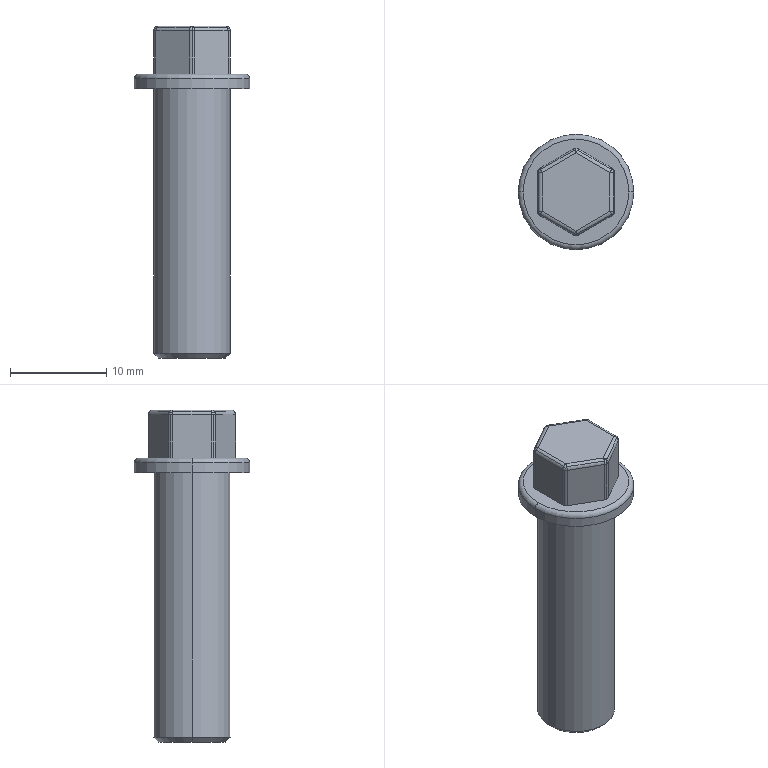Part | SolidWorks | features BaseBody 1 | 1 solid | 54 faces | box 12 x 12 x 34.5 mm | volume 1847 mm3 | cylinder 28 | sphere 12 | plane 10 | torus 2 | cone 2 | commonest cylinder face diameters 1 x24 8 x2 12 x2
STEP:
#1=CARTESIAN_POINT('',(-3.947,2.021,6.224));
#2=VERTEX_POINT('',#1);
#3=CARTESIAN_POINT('',(-4.,2.021,6.));
#4=VERTEX_POINT('',#3);
#5=CARTESIAN_POINT('',(-3.5,2.021,6.));
#6=DIRECTION('',(0.,-1.,0.));
#7=DIRECTION('',(0.,0.,1.));
#8=AXIS2_PLACEMENT_3D('',#5,#6,#7);
#9=CIRCLE('',#8,0.5);
#10=EDGE_CURVE('',#2,#4,#9,.T.);
#11=ORIENTED_EDGE('',*,*,#10,.F.);
#12=CARTESIAN_POINT('',(-3.724,2.408,6.224));
#13=VERTEX_POINT('',#12);
#14=CARTESIAN_POINT('',(-3.5,2.021,6.));
#15=DIRECTION('',(-0.433,0.25,-0.866));
#16=DIRECTION('',(-0.8944,0.,0.4472));
#17=AXIS2_PLACEMENT_3D('',#14,#15,#16);
#18=CIRCLE('',#17,0.5);
#19=EDGE_CURVE('',#2,#13,#18,.T.);
#20=ORIENTED_EDGE('',*,*,#19,.T.);
#21=CARTESIAN_POINT('',(-3.75,2.454,6.));
#22=VERTEX_POINT('',#21);
#23=CARTESIAN_POINT('',(-3.5,2.021,6.));
#24=DIRECTION('',(0.866,0.5,0.));
#25=DIRECTION('',(-0.5,0.866,0.));
#26=AXIS2_PLACEMENT_3D('',#23,#24,#25);
#27=CIRCLE('',#26,0.5);
#28=EDGE_CURVE('',#22,#13,#27,.T.);
#29=ORIENTED_EDGE('',*,*,#28,.F.);
#30=CARTESIAN_POINT('',(-3.933,2.271,6.));
#31=VERTEX_POINT('',#30);
#32=CARTESIAN_POINT('',(-3.5,2.021,6.));
#33=DIRECTION('',(0.,0.,-1.));
#34=DIRECTION('',(-1.,0.,0.));
#35=AXIS2_PLACEMENT_3D('',#32,#33,#34);
#36=CIRCLE('',#35,0.5);
#37=EDGE_CURVE('',#31,#22,#36,.T.);
#38=ORIENTED_EDGE('',*,*,#37,.F.);
#39=CARTESIAN_POINT('',(-3.5,2.021,6.));
#40=DIRECTION('',(0.,0.,-1.));
#41=DIRECTION('',(-1.,0.,0.));
#42=AXIS2_PLACEMENT_3D('',#39,#40,#41);
#43=CIRCLE('',#42,0.5);
#44=EDGE_CURVE('',#4,#31,#43,.T.);
#45=ORIENTED_EDGE('',*,*,#44,.F.);
#46=EDGE_LOOP('',(#11,#20,#29,#38,#45));
#47=FACE_OUTER_BOUND('',#46,.T.);
#48=CARTESIAN_POINT('',(-3.5,2.021,6.));
#49=DIRECTION('',(0.433,-0.25,0.866));
#50=DIRECTION('',(-0.75,0.433,0.5));
#51=AXIS2_PLACEMENT_3D('',#48,#49,#50);
#52=SPHERICAL_SURFACE('',#51,0.5);
#53=ADVANCED_FACE('',(#47),#52,.T.);
#54=ORIENTED_EDGE('',*,*,#44,.T.);
#55=CARTESIAN_POINT('',(-3.933,2.271,1.5));
#56=VERTEX_POINT('',#55);
#57=CARTESIAN_POINT('',(-3.933,2.271,1.5));
#58=DIRECTION('',(0.,0.,-1.));
#59=VECTOR('',#58,1000.);
#60=LINE('',#57,#59);
#61=EDGE_CURVE('',#31,#56,#60,.T.);
#62=ORIENTED_EDGE('',*,*,#61,.T.);
#63=CARTESIAN_POINT('',(-4.,2.021,1.5));
#64=VERTEX_POINT('',#63);
#65=CARTESIAN_POINT('',(-3.5,2.021,1.5));
#66=DIRECTION('',(0.,0.,1.));
#67=DIRECTION('',(-0.866,0.5,0.));
#68=AXIS2_PLACEMENT_3D('',#65,#66,#67);
#69=CIRCLE('',#68,0.5);
#70=EDGE_CURVE('',#56,#64,#69,.T.);
#71=ORIENTED_EDGE('',*,*,#70,.T.);
#72=CARTESIAN_POINT('',(-4.,2.021,1.5));
#73=DIRECTION('',(0.,0.,1.));
#74=VECTOR('',#73,1000.);
#75=LINE('',#72,#74);
#76=EDGE_CURVE('',#64,#4,#75,.T.);
#77=ORIENTED_EDGE('',*,*,#76,.T.);
#78=EDGE_LOOP('',(#54,#62,#71,#77));
#79=FACE_OUTER_BOUND('',#78,.T.);
#80=CARTESIAN_POINT('',(-3.5,2.021,1.5));
#81=DIRECTION('',(0.,0.,-1.));
#82=DIRECTION('',(-0.866,0.5,0.));
#83=AXIS2_PLACEMENT_3D('',#80,#81,#82);
#84=CYLINDRICAL_SURFACE('',#83,0.5);
#85=ADVANCED_FACE('',(#79),#84,.T.);
#86=CARTESIAN_POINT('',(-3.724,-2.408,6.224));
#87=VERTEX_POINT('',#86);
#88=CARTESIAN_POINT('',(-3.75,-2.454,6.));
#89=VERTEX_POINT('',#88);
#90=CARTESIAN_POINT('',(-3.5,-2.021,6.));
#91=DIRECTION('',(0.866,-0.5,0.));
#92=DIRECTION('',(0.,0.,1.));
#93=AXIS2_PLACEMENT_3D('',#90,#91,#92);
#94=CIRCLE('',#93,0.5);
#95=EDGE_CURVE('',#87,#89,#94,.T.);
#96=ORIENTED_EDGE('',*,*,#95,.F.);
#97=CARTESIAN_POINT('',(-3.947,-2.021,6.224));
#98=VERTEX_POINT('',#97);
#99=CARTESIAN_POINT('',(-3.5,-2.021,6.));
#100=DIRECTION('',(-0.433,-0.25,-0.866));
#101=DIRECTION('',(-0.8944,0.,0.4472));
#102=AXIS2_PLACEMENT_3D('',#99,#100,#101);
#103=CIRCLE('',#102,0.5);
#104=EDGE_CURVE('',#87,#98,#103,.T.);
#105=ORIENTED_EDGE('',*,*,#104,.T.);
#106=CARTESIAN_POINT('',(-4.,-2.021,6.));
#107=VERTEX_POINT('',#106);
#108=CARTESIAN_POINT('',(-3.5,-2.021,6.));
#109=DIRECTION('',(0.,1.,0.));
#110=DIRECTION('',(-1.,0.,0.));
#111=AXIS2_PLACEMENT_3D('',#108,#109,#110);
#112=CIRCLE('',#111,0.5);
#113=EDGE_CURVE('',#107,#98,#112,.T.);
#114=ORIENTED_EDGE('',*,*,#113,.F.);
#115=CARTESIAN_POINT('',(-3.933,-2.271,6.));
#116=VERTEX_POINT('',#115);
#117=CARTESIAN_POINT('',(-3.5,-2.021,6.));
#118=DIRECTION('',(0.,0.,-1.));
#119=DIRECTION('',(-0.5,-0.866,0.));
#120=AXIS2_PLACEMENT_3D('',#117,#118,#119);
#121=CIRCLE('',#120,0.5);
#122=EDGE_CURVE('',#116,#107,#121,.T.);
#123=ORIENTED_EDGE('',*,*,#122,.F.);
#124=CARTESIAN_POINT('',(-3.5,-2.021,6.));
#125=DIRECTION('',(0.,0.,-1.));
#126=DIRECTION('',(-0.5,-0.866,0.));
#127=AXIS2_PLACEMENT_3D('',#124,#125,#126);
#128=CIRCLE('',#127,0.5);
#129=EDGE_CURVE('',#89,#116,#128,.T.);
#130=ORIENTED_EDGE('',*,*,#129,.F.);
#131=EDGE_LOOP('',(#96,#105,#114,#123,#130));
#132=FACE_OUTER_BOUND('',#131,.T.);
#133=CARTESIAN_POINT('',(-3.5,-2.021,6.));
#134=DIRECTION('',(0.433,0.25,0.866));
#135=DIRECTION('',(-0.75,-0.433,0.5));
#136=AXIS2_PLACEMENT_3D('',#133,#134,#135);
#137=SPHERICAL_SURFACE('',#136,0.5);
#138=ADVANCED_FACE('',(#132),#137,.T.);
#139=ORIENTED_EDGE('',*,*,#129,.T.);
#140=CARTESIAN_POINT('',(-3.933,-2.271,1.5));
#141=VERTEX_POINT('',#140);
#142=CARTESIAN_POINT('',(-3.933,-2.271,1.5));
#143=DIRECTION('',(0.,0.,-1.));
#144=VECTOR('',#143,1000.);
#145=LINE('',#142,#144);
#146=EDGE_CURVE('',#116,#141,#145,.T.);
#147=ORIENTED_EDGE('',*,*,#146,.T.);
#148=CARTESIAN_POINT('',(-3.75,-2.454,1.5));
#149=VERTEX_POINT('',#148);
#150=CARTESIAN_POINT('',(-3.5,-2.021,1.5));
#151=DIRECTION('',(0.,0.,1.));
#152=DIRECTION('',(-0.866,-0.5,0.));
#153=AXIS2_PLACEMENT_3D('',#150,#151,#152);
#154=CIRCLE('',#153,0.5);
#155=EDGE_CURVE('',#141,#149,#154,.T.);
#156=ORIENTED_EDGE('',*,*,#155,.T.);
#157=CARTESIAN_POINT('',(-3.75,-2.454,1.5));
#158=DIRECTION('',(0.,0.,1.));
#159=VECTOR('',#158,1000.);
#160=LINE('',#157,#159);
#161=EDGE_CURVE('',#149,#89,#160,.T.);
#162=ORIENTED_EDGE('',*,*,#161,.T.);
#163=EDGE_LOOP('',(#139,#147,#156,#162));
#164=FACE_OUTER_BOUND('',#163,.T.);
#165=CARTESIAN_POINT('',(-3.5,-2.021,1.5));
#166=DIRECTION('',(0.,0.,-1.));
#167=DIRECTION('',(-0.866,-0.5,0.));
#168=AXIS2_PLACEMENT_3D('',#165,#166,#167);
#169=CYLINDRICAL_SURFACE('',#168,0.5);
#170=ADVANCED_FACE('',(#164),#169,.T.);
#171=CARTESIAN_POINT('',(0.,4.041,6.5));
#172=VERTEX_POINT('',#171);
#173=CARTESIAN_POINT('',(-0.1768,4.348,6.354));
#174=VERTEX_POINT('',#173);
#175=CARTESIAN_POINT('',(0.,4.041,6.));
#176=DIRECTION('',(-0.866,-0.5,0.));
#177=DIRECTION('',(0.,0.,1.));
#178=AXIS2_PLACEMENT_3D('',#175,#176,#177);
#179=CIRCLE('',#178,0.5);
#180=EDGE_CURVE('',#172,#174,#179,.T.);
#181=ORIENTED_EDGE('',*,*,#180,.F.);
#182=CARTESIAN_POINT('',(0.,4.541,6.));
#183=VERTEX_POINT('',#182);
#184=CARTESIAN_POINT('',(0.,4.041,6.));
#185=DIRECTION('',(-1.,0.,0.));
#186=DIRECTION('',(0.,-1.,0.));
#187=AXIS2_PLACEMENT_3D('',#184,#185,#186);
#188=CIRCLE('',#187,0.5);
#189=EDGE_CURVE('',#172,#183,#188,.T.);
#190=ORIENTED_EDGE('',*,*,#189,.T.);
#191=CARTESIAN_POINT('',(-0.25,4.474,6.));
#192=VERTEX_POINT('',#191);
#193=CARTESIAN_POINT('',(0.,4.041,6.));
#194=DIRECTION('',(0.,0.,-1.));
#195=DIRECTION('',(-0.5,0.866,0.));
#196=AXIS2_PLACEMENT_3D('',#193,#194,#195);
#197=CIRCLE('',#196,0.5);
#198=EDGE_CURVE('',#192,#183,#197,.T.);
#199=ORIENTED_EDGE('',*,*,#198,.F.);
#200=CARTESIAN_POINT('',(0.,4.041,6.));
#201=DIRECTION('',(-0.866,-0.5,0.));
#202=DIRECTION('',(0.,0.,1.));
#203=AXIS2_PLACEMENT_3D('',#200,#201,#202);
#204=CIRCLE('',#203,0.5);
#205=EDGE_CURVE('',#174,#192,#204,.T.);
#206=ORIENTED_EDGE('',*,*,#205,.F.);
#207=EDGE_LOOP('',(#181,#190,#199,#206));
#208=FACE_OUTER_BOUND('',#207,.T.);
#209=CARTESIAN_POINT('',(0.,4.041,6.));
#210=DIRECTION('',(1.,0.,0.));
#211=DIRECTION('',(0.,0.866,0.5));
#212=AXIS2_PLACEMENT_3D('',#209,#210,#211);
#213=SPHERICAL_SURFACE('',#212,0.5);
#214=ADVANCED_FACE('',(#208),#213,.T.);
#215=ORIENTED_EDGE('',*,*,#198,.T.);
#216=CARTESIAN_POINT('',(0.,4.541,1.5));
#217=VERTEX_POINT('',#216);
#218=CARTESIAN_POINT('',(0.,4.541,1.5));
#219=DIRECTION('',(0.,0.,-1.));
#220=VECTOR('',#219,1000.);
#221=LINE('',#218,#220);
#222=EDGE_CURVE('',#183,#217,#221,.T.);
#223=ORIENTED_EDGE('',*,*,#222,.T.);
#224=CARTESIAN_POINT('',(-0.25,4.474,1.5));
#225=VERTEX_POINT('',#224);
#226=CARTESIAN_POINT('',(0.,4.041,1.5));
#227=DIRECTION('',(0.,0.,1.));
#228=DIRECTION('',(0.,1.,0.));
#229=AXIS2_PLACEMENT_3D('',#226,#227,#228);
#230=CIRCLE('',#229,0.5);
#231=EDGE_CURVE('',#217,#225,#230,.T.);
#232=ORIENTED_EDGE('',*,*,#231,.T.);
#233=CARTESIAN_POINT('',(-0.25,4.474,1.5));
#234=DIRECTION('',(0.,0.,1.));
#235=VECTOR('',#234,1000.);
#236=LINE('',#233,#235);
#237=EDGE_CURVE('',#225,#192,#236,.T.);
#238=ORIENTED_EDGE('',*,*,#237,.T.);
#239=EDGE_LOOP('',(#215,#223,#232,#238));
#240=FACE_OUTER_BOUND('',#239,.T.);
#241=CARTESIAN_POINT('',(0.,4.041,1.5));
#242=DIRECTION('',(0.,0.,-1.));
#243=DIRECTION('',(0.,1.,0.));
#244=AXIS2_PLACEMENT_3D('',#241,#242,#243);
#245=CYLINDRICAL_SURFACE('',#244,0.5);
#246=ADVANCED_FACE('',(#240),#245,.T.);
#247=ORIENTED_EDGE('',*,*,#28,.T.);
#248=CARTESIAN_POINT('',(-3.677,2.327,6.354));
#249=VERTEX_POINT('',#248);
#250=CARTESIAN_POINT('',(-3.5,2.021,6.));
#251=DIRECTION('',(0.866,0.5,0.));
#252=DIRECTION('',(-0.5,0.866,0.));
#253=AXIS2_PLACEMENT_3D('',#250,#251,#252);
#254=CIRCLE('',#253,0.5);
#255=EDGE_CURVE('',#13,#249,#254,.T.);
#256=ORIENTED_EDGE('',*,*,#255,.T.);
#257=CARTESIAN_POINT('',(-0.9268,3.915,6.354));
#258=DIRECTION('',(0.866,0.5,0.));
#259=VECTOR('',#258,1000.);
#260=LINE('',#257,#259);
#261=EDGE_CURVE('',#249,#174,#260,.T.);
#262=ORIENTED_EDGE('',*,*,#261,.T.);
#263=ORIENTED_EDGE('',*,*,#205,.T.);
#264=CARTESIAN_POINT('',(-1.,4.041,6.));
#265=DIRECTION('',(-0.866,-0.5,0.));
#266=VECTOR('',#265,1000.);
#267=LINE('',#264,#266);
#268=EDGE_CURVE('',#192,#22,#267,.T.);
#269=ORIENTED_EDGE('',*,*,#268,.T.);
#270=EDGE_LOOP('',(#247,#256,#262,#263,#269));
#271=FACE_OUTER_BOUND('',#270,.T.);
#272=CARTESIAN_POINT('',(-0.75,3.608,6.));
#273=DIRECTION('',(0.866,0.5,0.));
#274=DIRECTION('',(-0.3536,0.6124,0.7071));
#275=AXIS2_PLACEMENT_3D('',#272,#273,#274);
#276=CYLINDRICAL_SURFACE('',#275,0.5);
#277=ADVANCED_FACE('',(#271),#276,.T.);
#278=CARTESIAN_POINT('',(0.,-4.541,6.));
#279=VERTEX_POINT('',#278);
#280=CARTESIAN_POINT('',(-0.25,-4.474,6.));
#281=VERTEX_POINT('',#280);
#282=CARTESIAN_POINT('',(0.,-4.041,6.));
#283=DIRECTION('',(0.,0.,-1.));
#284=DIRECTION('',(0.5,-0.866,0.));
#285=AXIS2_PLACEMENT_3D('',#282,#283,#284);
#286=CIRCLE('',#285,0.5);
#287=EDGE_CURVE('',#279,#281,#286,.T.);
#288=ORIENTED_EDGE('',*,*,#287,.F.);
#289=CARTESIAN_POINT('',(0.,-4.041,6.5));
#290=VERTEX_POINT('',#289);
#291=CARTESIAN_POINT('',(0.,-4.041,6.));
#292=DIRECTION('',(-1.,0.,0.));
#293=DIRECTION('',(0.,-1.,0.));
#294=AXIS2_PLACEMENT_3D('',#291,#292,#293);
#295=CIRCLE('',#294,0.5);
#296=EDGE_CURVE('',#279,#290,#295,.T.);
#297=ORIENTED_EDGE('',*,*,#296,.T.);
#298=CARTESIAN_POINT('',(-0.1768,-4.348,6.354));
#299=VERTEX_POINT('',#298);
#300=CARTESIAN_POINT('',(0.,-4.041,6.));
#301=DIRECTION('',(-0.866,0.5,0.));
#302=DIRECTION('',(-0.5,-0.866,0.));
#303=AXIS2_PLACEMENT_3D('',#300,#301,#302);
#304=CIRCLE('',#303,0.5);
#305=EDGE_CURVE('',#299,#290,#304,.T.);
#306=ORIENTED_EDGE('',*,*,#305,.F.);
#307=CARTESIAN_POINT('',(0.,-4.041,6.));
#308=DIRECTION('',(-0.866,0.5,0.));
#309=DIRECTION('',(-0.5,-0.866,0.));
#310=AXIS2_PLACEMENT_3D('',#307,#308,#309);
#311=CIRCLE('',#310,0.5);
#312=EDGE_CURVE('',#281,#299,#311,.T.);
#313=ORIENTED_EDGE('',*,*,#312,.F.);
#314=EDGE_LOOP('',(#288,#297,#306,#313));
#315=FACE_OUTER_BOUND('',#314,.T.);
#316=CARTESIAN_POINT('',(0.,-4.041,6.));
#317=DIRECTION('',(1.,0.,0.));
#318=DIRECTION('',(0.,-0.866,0.5));
#319=AXIS2_PLACEMENT_3D('',#316,#317,#318);
#320=SPHERICAL_SURFACE('',#319,0.5);
#321=ADVANCED_FACE('',(#315),#320,.T.);
#322=CARTESIAN_POINT('',(0.25,-4.474,6.));
#323=VERTEX_POINT('',#322);
#324=CARTESIAN_POINT('',(0.,-4.041,6.));
#325=DIRECTION('',(0.,0.,-1.));
#326=DIRECTION('',(0.5,-0.866,0.));
#327=AXIS2_PLACEMENT_3D('',#324,#325,#326);
#328=CIRCLE('',#327,0.5);
#329=EDGE_CURVE('',#323,#279,#328,.T.);
#330=ORIENTED_EDGE('',*,*,#329,.T.);
#331=CARTESIAN_POINT('',(0.,-4.541,1.5));
#332=VERTEX_POINT('',#331);
#333=CARTESIAN_POINT('',(0.,-4.541,1.5));
#334=DIRECTION('',(0.,0.,-1.));
#335=VECTOR('',#334,1000.);
#336=LINE('',#333,#335);
#337=EDGE_CURVE('',#279,#332,#336,.T.);
#338=ORIENTED_EDGE('',*,*,#337,.T.);
#339=CARTESIAN_POINT('',(0.25,-4.474,1.5));
#340=VERTEX_POINT('',#339);
#341=CARTESIAN_POINT('',(0.,-4.041,1.5));
#342=DIRECTION('',(0.,0.,1.));
#343=DIRECTION('',(0.,-1.,0.));
#344=AXIS2_PLACEMENT_3D('',#341,#342,#343);
#345=CIRCLE('',#344,0.5);
#346=EDGE_CURVE('',#332,#340,#345,.T.);
#347=ORIENTED_EDGE('',*,*,#346,.T.);
#348=CARTESIAN_POINT('',(0.25,-4.474,1.5));
#349=DIRECTION('',(0.,0.,1.));
#350=VECTOR('',#349,1000.);
#351=LINE('',#348,#350);
#352=EDGE_CURVE('',#340,#323,#351,.T.);
#353=ORIENTED_EDGE('',*,*,#352,.T.);
#354=EDGE_LOOP('',(#330,#338,#347,#353));
#355=FACE_OUTER_BOUND('',#354,.T.);
#356=CARTESIAN_POINT('',(0.,-4.041,1.5));
#357=DIRECTION('',(0.,0.,-1.));
#358=DIRECTION('',(0.,-1.,0.));
#359=AXIS2_PLACEMENT_3D('',#356,#357,#358);
#360=CYLINDRICAL_SURFACE('',#359,0.5);
#361=ADVANCED_FACE('',(#355),#360,.T.);
#362=CARTESIAN_POINT('',(3.724,2.408,6.224));
#363=VERTEX_POINT('',#362);
#364=CARTESIAN_POINT('',(3.75,2.454,6.));
#365=VERTEX_POINT('',#364);
#366=CARTESIAN_POINT('',(3.5,2.021,6.));
#367=DIRECTION('',(-0.866,0.5,0.));
#368=DIRECTION('',(0.,0.,1.));
#369=AXIS2_PLACEMENT_3D('',#366,#367,#368);
#370=CIRCLE('',#369,0.5);
#371=EDGE_CURVE('',#363,#365,#370,.T.);
#372=ORIENTED_EDGE('',*,*,#371,.F.);
#373=CARTESIAN_POINT('',(3.947,2.021,6.224));
#374=VERTEX_POINT('',#373);
#375=CARTESIAN_POINT('',(3.5,2.021,6.));
#376=DIRECTION('',(0.433,0.25,-0.866));
#377=DIRECTION('',(-0.8944,0.,-0.4472));
#378=AXIS2_PLACEMENT_3D('',#375,#376,#377);
#379=CIRCLE('',#378,0.5);
#380=EDGE_CURVE('',#363,#374,#379,.T.);
#381=ORIENTED_EDGE('',*,*,#380,.T.);
#382=CARTESIAN_POINT('',(4.,2.021,6.));
#383=VERTEX_POINT('',#382);
#384=CARTESIAN_POINT('',(3.5,2.021,6.));
#385=DIRECTION('',(0.,-1.,0.));
#386=DIRECTION('',(1.,0.,0.));
#387=AXIS2_PLACEMENT_3D('',#384,#385,#386);
#388=CIRCLE('',#387,0.5);
#389=EDGE_CURVE('',#383,#374,#388,.T.);
#390=ORIENTED_EDGE('',*,*,#389,.F.);
#391=CARTESIAN_POINT('',(3.933,2.271,6.));
#392=VERTEX_POINT('',#391);
#393=CARTESIAN_POINT('',(3.5,2.021,6.));
#394=DIRECTION('',(0.,0.,-1.));
#395=DIRECTION('',(0.5,0.866,0.));
#396=AXIS2_PLACEMENT_3D('',#393,#394,#395);
#397=CIRCLE('',#396,0.5);
#398=EDGE_CURVE('',#392,#383,#397,.T.);
#399=ORIENTED_EDGE('',*,*,#398,.F.);
#400=CARTESIAN_POINT('',(3.5,2.021,6.));
#401=DIRECTION('',(0.,0.,-1.));
#402=DIRECTION('',(0.5,0.866,0.));
#403=AXIS2_PLACEMENT_3D('',#400,#401,#402);
#404=CIRCLE('',#403,0.5);
#405=EDGE_CURVE('',#365,#392,#404,.T.);
#406=ORIENTED_EDGE('',*,*,#405,.F.);
#407=EDGE_LOOP('',(#372,#381,#390,#399,#406));
#408=FACE_OUTER_BOUND('',#407,.T.);
#409=CARTESIAN_POINT('',(3.5,2.021,6.));
#410=DIRECTION('',(-0.433,-0.25,0.866));
#411=DIRECTION('',(0.75,0.433,0.5));
#412=AXIS2_PLACEMENT_3D('',#409,#410,#411);
#413=SPHERICAL_SURFACE('',#412,0.5);
#414=ADVANCED_FACE('',(#408),#413,.T.);
#415=ORIENTED_EDGE('',*,*,#405,.T.);
#416=CARTESIAN_POINT('',(3.933,2.271,1.5));
#417=VERTEX_POINT('',#416);
#418=CARTESIAN_POINT('',(3.933,2.271,1.5));
#419=DIRECTION('',(0.,0.,-1.));
#420=VECTOR('',#419,1000.);
#421=LINE('',#418,#420);
#422=EDGE_CURVE('',#392,#417,#421,.T.);
#423=ORIENTED_EDGE('',*,*,#422,.T.);
#424=CARTESIAN_POINT('',(3.75,2.454,1.5));
#425=VERTEX_POINT('',#424);
#426=CARTESIAN_POINT('',(3.5,2.021,1.5));
#427=DIRECTION('',(0.,0.,1.));
#428=DIRECTION('',(0.866,0.5,0.));
#429=AXIS2_PLACEMENT_3D('',#426,#427,#428);
#430=CIRCLE('',#429,0.5);
#431=EDGE_CURVE('',#417,#425,#430,.T.);
#432=ORIENTED_EDGE('',*,*,#431,.T.);
#433=CARTESIAN_POINT('',(3.75,2.454,1.5));
#434=DIRECTION('',(0.,0.,1.));
#435=VECTOR('',#434,1000.);
#436=LINE('',#433,#435);
#437=EDGE_CURVE('',#425,#365,#436,.T.);
#438=ORIENTED_EDGE('',*,*,#437,.T.);
#439=EDGE_LOOP('',(#415,#423,#432,#438));
#440=FACE_OUTER_BOUND('',#439,.T.);
#441=CARTESIAN_POINT('',(3.5,2.021,1.5));
#442=DIRECTION('',(0.,0.,-1.));
#443=DIRECTION('',(0.866,0.5,0.));
#444=AXIS2_PLACEMENT_3D('',#441,#442,#443);
#445=CYLINDRICAL_SURFACE('',#444,0.5);
#446=ADVANCED_FACE('',(#440),#445,.T.);
#447=CARTESIAN_POINT('',(0.25,4.474,6.));
#448=VERTEX_POINT('',#447);
#449=CARTESIAN_POINT('',(0.1768,4.348,6.354));
#450=VERTEX_POINT('',#449);
#451=CARTESIAN_POINT('',(0.,4.041,6.));
#452=DIRECTION('',(0.866,-0.5,0.));
#453=DIRECTION('',(0.5,0.866,0.));
#454=AXIS2_PLACEMENT_3D('',#451,#452,#453);
#455=CIRCLE('',#454,0.5);
#456=EDGE_CURVE('',#448,#450,#455,.T.);
#457=ORIENTED_EDGE('',*,*,#456,.T.);
#458=CARTESIAN_POINT('',(3.677,2.327,6.354));
#459=VERTEX_POINT('',#458);
#460=CARTESIAN_POINT('',(2.927,2.76,6.354));
#461=DIRECTION('',(0.866,-0.5,0.));
#462=VECTOR('',#461,1000.);
#463=LINE('',#460,#462);
#464=EDGE_CURVE('',#450,#459,#463,.T.);
#465=ORIENTED_EDGE('',*,*,#464,.T.);
#466=CARTESIAN_POINT('',(3.5,2.021,6.));
#467=DIRECTION('',(-0.866,0.5,0.));
#468=DIRECTION('',(0.,0.,1.));
#469=AXIS2_PLACEMENT_3D('',#466,#467,#468);
#470=CIRCLE('',#469,0.5);
#471=EDGE_CURVE('',#459,#363,#470,.T.);
#472=ORIENTED_EDGE('',*,*,#471,.T.);
#473=ORIENTED_EDGE('',*,*,#371,.T.);
#474=CARTESIAN_POINT('',(3.,2.887,6.));
#475=DIRECTION('',(-0.866,0.5,0.));
#476=VECTOR('',#475,1000.);
#477=LINE('',#474,#476);
#478=EDGE_CURVE('',#365,#448,#477,.T.);
#479=ORIENTED_EDGE('',*,*,#478,.T.);
#480=EDGE_LOOP('',(#457,#465,#472,#473,#479));
#481=FACE_OUTER_BOUND('',#480,.T.);
#482=CARTESIAN_POINT('',(2.75,2.454,6.));
#483=DIRECTION('',(0.866,-0.5,0.));
#484=DIRECTION('',(0.3536,0.6124,0.7071));
#485=AXIS2_PLACEMENT_3D('',#482,#483,#484);
#486=CYLINDRICAL_SURFACE('',#485,0.5);
#487=ADVANCED_FACE('',(#481),#486,.T.);
#488=CARTESIAN_POINT('',(3.947,-2.021,6.224));
#489=VERTEX_POINT('',#488);
#490=CARTESIAN_POINT('',(4.,-2.021,6.));
#491=VERTEX_POINT('',#490);
#492=CARTESIAN_POINT('',(3.5,-2.021,6.));
#493=DIRECTION('',(0.,1.,0.));
#494=DIRECTION('',(0.,0.,1.));
#495=AXIS2_PLACEMENT_3D('',#492,#493,#494);
#496=CIRCLE('',#495,0.5);
#497=EDGE_CURVE('',#489,#491,#496,.T.);
#498=ORIENTED_EDGE('',*,*,#497,.F.);
#499=CARTESIAN_POINT('',(3.724,-2.408,6.224));
#500=VERTEX_POINT('',#499);
#501=CARTESIAN_POINT('',(3.5,-2.021,6.));
#502=DIRECTION('',(0.433,-0.25,-0.866));
#503=DIRECTION('',(-0.8944,0.,-0.4472));
#504=AXIS2_PLACEMENT_3D('',#501,#502,#503);
#505=CIRCLE('',#504,0.5);
#506=EDGE_CURVE('',#489,#500,#505,.T.);
#507=ORIENTED_EDGE('',*,*,#506,.T.);
#508=CARTESIAN_POINT('',(3.75,-2.454,6.));
#509=VERTEX_POINT('',#508);
#510=CARTESIAN_POINT('',(3.5,-2.021,6.));
#511=DIRECTION('',(-0.866,-0.5,0.));
#512=DIRECTION('',(0.5,-0.866,0.));
#513=AXIS2_PLACEMENT_3D('',#510,#511,#512);
#514=CIRCLE('',#513,0.5);
#515=EDGE_CURVE('',#509,#500,#514,.T.);
#516=ORIENTED_EDGE('',*,*,#515,.F.);
#517=CARTESIAN_POINT('',(3.933,-2.271,6.));
#518=VERTEX_POINT('',#517);
#519=CARTESIAN_POINT('',(3.5,-2.021,6.));
#520=DIRECTION('',(0.,0.,-1.));
#521=DIRECTION('',(1.,0.,0.));
#522=AXIS2_PLACEMENT_3D('',#519,#520,#521);
#523=CIRCLE('',#522,0.5);
#524=EDGE_CURVE('',#518,#509,#523,.T.);
#525=ORIENTED_EDGE('',*,*,#524,.F.);
#526=CARTESIAN_POINT('',(3.5,-2.021,6.));
#527=DIRECTION('',(0.,0.,-1.));
#528=DIRECTION('',(1.,0.,0.));
#529=AXIS2_PLACEMENT_3D('',#526,#527,#528);
#530=CIRCLE('',#529,0.5);
#531=EDGE_CURVE('',#491,#518,#530,.T.);
#532=ORIENTED_EDGE('',*,*,#531,.F.);
#533=EDGE_LOOP('',(#498,#507,#516,#525,#532));
#534=FACE_OUTER_BOUND('',#533,.T.);
#535=CARTESIAN_POINT('',(3.5,-2.021,6.));
#536=DIRECTION('',(-0.433,0.25,0.866));
#537=DIRECTION('',(0.75,-0.433,0.5));
#538=AXIS2_PLACEMENT_3D('',#535,#536,#537);
#539=SPHERICAL_SURFACE('',#538,0.5);
#540=ADVANCED_FACE('',(#534),#539,.T.);
#541=ORIENTED_EDGE('',*,*,#531,.T.);
#542=CARTESIAN_POINT('',(3.933,-2.271,1.5));
#543=VERTEX_POINT('',#542);
#544=CARTESIAN_POINT('',(3.933,-2.271,1.5));
#545=DIRECTION('',(0.,0.,-1.));
#546=VECTOR('',#545,1000.);
#547=LINE('',#544,#546);
#548=EDGE_CURVE('',#518,#543,#547,.T.);
#549=ORIENTED_EDGE('',*,*,#548,.T.);
#550=CARTESIAN_POINT('',(4.,-2.021,1.5));
#551=VERTEX_POINT('',#550);
#552=CARTESIAN_POINT('',(3.5,-2.021,1.5));
#553=DIRECTION('',(0.,0.,1.));
#554=DIRECTION('',(0.866,-0.5,0.));
#555=AXIS2_PLACEMENT_3D('',#552,#553,#554);
#556=CIRCLE('',#555,0.5);
#557=EDGE_CURVE('',#543,#551,#556,.T.);
#558=ORIENTED_EDGE('',*,*,#557,.T.);
#559=CARTESIAN_POINT('',(4.,-2.021,1.5));
#560=DIRECTION('',(0.,0.,1.));
#561=VECTOR('',#560,1000.);
#562=LINE('',#559,#561);
#563=EDGE_CURVE('',#551,#491,#562,.T.);
#564=ORIENTED_EDGE('',*,*,#563,.T.);
#565=EDGE_LOOP('',(#541,#549,#558,#564));
#566=FACE_OUTER_BOUND('',#565,.T.);
#567=CARTESIAN_POINT('',(3.5,-2.021,1.5));
#568=DIRECTION('',(0.,0.,-1.));
#569=DIRECTION('',(0.866,-0.5,0.));
#570=AXIS2_PLACEMENT_3D('',#567,#568,#569);
#571=CYLINDRICAL_SURFACE('',#570,0.5);
#572=ADVANCED_FACE('',(#566),#571,.T.);
#573=ORIENTED_EDGE('',*,*,#389,.T.);
#574=CARTESIAN_POINT('',(3.854,2.021,6.354));
#575=VERTEX_POINT('',#574);
#576=CARTESIAN_POINT('',(3.5,2.021,6.));
#577=DIRECTION('',(0.,-1.,0.));
#578=DIRECTION('',(1.,0.,0.));
#579=AXIS2_PLACEMENT_3D('',#576,#577,#578);
#580=CIRCLE('',#579,0.5);
#581=EDGE_CURVE('',#374,#575,#580,.T.);
#582=ORIENTED_EDGE('',*,*,#581,.T.);
#583=CARTESIAN_POINT('',(3.854,-2.021,6.354));
#584=VERTEX_POINT('',#583);
#585=CARTESIAN_POINT('',(3.854,-1.155,6.354));
#586=DIRECTION('',(0.,-1.,0.));
#587=VECTOR('',#586,1000.);
#588=LINE('',#585,#587);
#589=EDGE_CURVE('',#575,#584,#588,.T.);
#590=ORIENTED_EDGE('',*,*,#589,.T.);
#591=CARTESIAN_POINT('',(3.5,-2.021,6.));
#592=DIRECTION('',(0.,1.,0.));
#593=DIRECTION('',(0.,0.,1.));
#594=AXIS2_PLACEMENT_3D('',#591,#592,#593);
#595=CIRCLE('',#594,0.5);
#596=EDGE_CURVE('',#584,#489,#595,.T.);
#597=ORIENTED_EDGE('',*,*,#596,.T.);
#598=ORIENTED_EDGE('',*,*,#497,.T.);
#599=CARTESIAN_POINT('',(4.,-1.155,6.));
#600=DIRECTION('',(0.,1.,0.));
#601=VECTOR('',#600,1000.);
#602=LINE('',#599,#601);
#603=EDGE_CURVE('',#491,#383,#602,.T.);
#604=ORIENTED_EDGE('',*,*,#603,.T.);
#605=EDGE_LOOP('',(#573,#582,#590,#597,#598,#604));
#606=FACE_OUTER_BOUND('',#605,.T.);
#607=CARTESIAN_POINT('',(3.5,-1.155,6.));
#608=DIRECTION('',(0.,-1.,0.));
#609=DIRECTION('',(0.7071,0.,0.7071));
#610=AXIS2_PLACEMENT_3D('',#607,#608,#609);
#611=CYLINDRICAL_SURFACE('',#610,0.5);
#612=ADVANCED_FACE('',(#606),#611,.T.);
#613=ORIENTED_EDGE('',*,*,#515,.T.);
#614=CARTESIAN_POINT('',(3.677,-2.327,6.354));
#615=VERTEX_POINT('',#614);
#616=CARTESIAN_POINT('',(3.5,-2.021,6.));
#617=DIRECTION('',(-0.866,-0.5,0.));
#618=DIRECTION('',(0.5,-0.866,0.));
#619=AXIS2_PLACEMENT_3D('',#616,#617,#618);
#620=CIRCLE('',#619,0.5);
#621=EDGE_CURVE('',#500,#615,#620,.T.);
#622=ORIENTED_EDGE('',*,*,#621,.T.);
#623=CARTESIAN_POINT('',(0.1768,-4.348,6.354));
#624=VERTEX_POINT('',#623);
#625=CARTESIAN_POINT('',(0.9268,-3.915,6.354));
#626=DIRECTION('',(-0.866,-0.5,0.));
#627=VECTOR('',#626,1000.);
#628=LINE('',#625,#627);
#629=EDGE_CURVE('',#615,#624,#628,.T.);
#630=ORIENTED_EDGE('',*,*,#629,.T.);
#631=CARTESIAN_POINT('',(0.,-4.041,6.));
#632=DIRECTION('',(0.866,0.5,0.));
#633=DIRECTION('',(0.,0.,1.));
#634=AXIS2_PLACEMENT_3D('',#631,#632,#633);
#635=CIRCLE('',#634,0.5);
#636=EDGE_CURVE('',#624,#323,#635,.T.);
#637=ORIENTED_EDGE('',*,*,#636,.T.);
#638=CARTESIAN_POINT('',(1.,-4.041,6.));
#639=DIRECTION('',(0.866,0.5,0.));
#640=VECTOR('',#639,1000.);
#641=LINE('',#638,#640);
#642=EDGE_CURVE('',#323,#509,#641,.T.);
#643=ORIENTED_EDGE('',*,*,#642,.T.);
#644=EDGE_LOOP('',(#613,#622,#630,#637,#643));
#645=FACE_OUTER_BOUND('',#644,.T.);
#646=CARTESIAN_POINT('',(0.75,-3.608,6.));
#647=DIRECTION('',(-0.866,-0.5,0.));
#648=DIRECTION('',(0.3536,-0.6124,0.7071));
#649=AXIS2_PLACEMENT_3D('',#646,#647,#648);
#650=CYLINDRICAL_SURFACE('',#649,0.5);
#651=ADVANCED_FACE('',(#645),#650,.T.);
#652=ORIENTED_EDGE('',*,*,#312,.T.);
#653=CARTESIAN_POINT('',(-3.677,-2.327,6.354));
#654=VERTEX_POINT('',#653);
#655=CARTESIAN_POINT('',(-2.927,-2.76,6.354));
#656=DIRECTION('',(-0.866,0.5,0.));
#657=VECTOR('',#656,1000.);
#658=LINE('',#655,#657);
#659=EDGE_CURVE('',#299,#654,#658,.T.);
#660=ORIENTED_EDGE('',*,*,#659,.T.);
#661=CARTESIAN_POINT('',(-3.5,-2.021,6.));
#662=DIRECTION('',(0.866,-0.5,0.));
#663=DIRECTION('',(0.,0.,1.));
#664=AXIS2_PLACEMENT_3D('',#661,#662,#663);
#665=CIRCLE('',#664,0.5);
#666=EDGE_CURVE('',#654,#87,#665,.T.);
#667=ORIENTED_EDGE('',*,*,#666,.T.);
#668=ORIENTED_EDGE('',*,*,#95,.T.);
#669=CARTESIAN_POINT('',(-3.,-2.887,6.));
#670=DIRECTION('',(0.866,-0.5,0.));
#671=VECTOR('',#670,1000.);
#672=LINE('',#669,#671);
#673=EDGE_CURVE('',#89,#281,#672,.T.);
#674=ORIENTED_EDGE('',*,*,#673,.T.);
#675=EDGE_LOOP('',(#652,#660,#667,#668,#674));
#676=FACE_OUTER_BOUND('',#675,.T.);
#677=CARTESIAN_POINT('',(-2.75,-2.454,6.));
#678=DIRECTION('',(-0.866,0.5,0.));
#679=DIRECTION('',(-0.3536,-0.6124,0.7071));
#680=AXIS2_PLACEMENT_3D('',#677,#678,#679);
#681=CYLINDRICAL_SURFACE('',#680,0.5);
#682=ADVANCED_FACE('',(#676),#681,.T.);
#683=ORIENTED_EDGE('',*,*,#113,.T.);
#684=CARTESIAN_POINT('',(-3.854,-2.021,6.354));
#685=VERTEX_POINT('',#684);
#686=CARTESIAN_POINT('',(-3.5,-2.021,6.));
#687=DIRECTION('',(0.,1.,0.));
#688=DIRECTION('',(-1.,0.,0.));
#689=AXIS2_PLACEMENT_3D('',#686,#687,#688);
#690=CIRCLE('',#689,0.5);
#691=EDGE_CURVE('',#98,#685,#690,.T.);
#692=ORIENTED_EDGE('',*,*,#691,.T.);
#693=CARTESIAN_POINT('',(-3.854,2.021,6.354));
#694=VERTEX_POINT('',#693);
#695=CARTESIAN_POINT('',(-3.854,1.155,6.354));
#696=DIRECTION('',(0.,1.,0.));
#697=VECTOR('',#696,1000.);
#698=LINE('',#695,#697);
#699=EDGE_CURVE('',#685,#694,#698,.T.);
#700=ORIENTED_EDGE('',*,*,#699,.T.);
#701=CARTESIAN_POINT('',(-3.5,2.021,6.));
#702=DIRECTION('',(0.,-1.,0.));
#703=DIRECTION('',(0.,0.,1.));
#704=AXIS2_PLACEMENT_3D('',#701,#702,#703);
#705=CIRCLE('',#704,0.5);
#706=EDGE_CURVE('',#694,#2,#705,.T.);
#707=ORIENTED_EDGE('',*,*,#706,.T.);
#708=ORIENTED_EDGE('',*,*,#10,.T.);
#709=CARTESIAN_POINT('',(-4.,1.155,6.));
#710=DIRECTION('',(0.,-1.,0.));
#711=VECTOR('',#710,1000.);
#712=LINE('',#709,#711);
#713=EDGE_CURVE('',#4,#107,#712,.T.);
#714=ORIENTED_EDGE('',*,*,#713,.T.);
#715=EDGE_LOOP('',(#683,#692,#700,#707,#708,#714));
#716=FACE_OUTER_BOUND('',#715,.T.);
#717=CARTESIAN_POINT('',(-3.5,1.155,6.));
#718=DIRECTION('',(0.,1.,0.));
#719=DIRECTION('',(-0.7071,0.,0.7071));
#720=AXIS2_PLACEMENT_3D('',#717,#718,#719);
#721=CYLINDRICAL_SURFACE('',#720,0.5);
#722=ADVANCED_FACE('',(#716),#721,.T.);
#723=CARTESIAN_POINT('',(6.,0.,1.));
#724=VERTEX_POINT('',#723);
#725=CARTESIAN_POINT('',(-6.,0.,1.));
#726=VERTEX_POINT('',#725);
#727=CARTESIAN_POINT('',(0.,0.,1.));
#728=DIRECTION('',(0.,0.,1.));
#729=DIRECTION('',(-1.,0.,0.));
#730=AXIS2_PLACEMENT_3D('',#727,#728,#729);
#731=CIRCLE('',#730,6.);
#732=EDGE_CURVE('',#724,#726,#731,.T.);
#733=ORIENTED_EDGE('',*,*,#732,.T.);
#734=CARTESIAN_POINT('',(-5.5,0.,1.5));
#735=VERTEX_POINT('',#734);
#736=CARTESIAN_POINT('',(-5.5,0.,1.));
#737=DIRECTION('',(0.,1.,0.));
#738=DIRECTION('',(-1.,0.,0.));
#739=AXIS2_PLACEMENT_3D('',#736,#737,#738);
#740=CIRCLE('',#739,0.5);
#741=EDGE_CURVE('',#726,#735,#740,.T.);
#742=ORIENTED_EDGE('',*,*,#741,.T.);
#743=CARTESIAN_POINT('',(5.5,0.,1.5));
#744=VERTEX_POINT('',#743);
#745=CARTESIAN_POINT('',(0.,0.,1.5));
#746=DIRECTION('',(0.,0.,-1.));
#747=DIRECTION('',(-1.,0.,0.));
#748=AXIS2_PLACEMENT_3D('',#745,#746,#747);
#749=CIRCLE('',#748,5.5);
#750=EDGE_CURVE('',#735,#744,#749,.T.);
#751=ORIENTED_EDGE('',*,*,#750,.T.);
#752=CARTESIAN_POINT('',(5.5,0.,1.));
#753=DIRECTION('',(0.,-1.,0.));
#754=DIRECTION('',(0.,0.,-1.));
#755=AXIS2_PLACEMENT_3D('',#752,#753,#754);
#756=CIRCLE('',#755,0.5);
#757=EDGE_CURVE('',#724,#744,#756,.T.);
#758=ORIENTED_EDGE('',*,*,#757,.F.);
#759=EDGE_LOOP('',(#733,#742,#751,#758));
#760=FACE_OUTER_BOUND('',#759,.T.);
#761=CARTESIAN_POINT('',(0.,0.,1.));
#762=DIRECTION('',(0.,0.,1.));
#763=DIRECTION('',(1.,0.,0.));
#764=AXIS2_PLACEMENT_3D('',#761,#762,#763);
#765=TOROIDAL_SURFACE('',#764,5.5,0.5);
#766=ADVANCED_FACE('',(#760),#765,.T.);
#767=ORIENTED_EDGE('',*,*,#732,.F.);
#768=CARTESIAN_POINT('',(6.,0.,0.));
#769=VERTEX_POINT('',#768);
#770=CARTESIAN_POINT('',(6.,0.,0.));
#771=DIRECTION('',(0.,0.,-1.));
#772=VECTOR('',#771,1000.);
#773=LINE('',#770,#772);
#774=EDGE_CURVE('',#724,#769,#773,.T.);
#775=ORIENTED_EDGE('',*,*,#774,.T.);
#776=CARTESIAN_POINT('',(-6.,0.,0.));
#777=VERTEX_POINT('',#776);
#778=CARTESIAN_POINT('',(0.,0.,0.));
#779=DIRECTION('',(0.,0.,-1.));
#780=DIRECTION('',(-1.,0.,0.));
#781=AXIS2_PLACEMENT_3D('',#778,#779,#780);
#782=CIRCLE('',#781,6.);
#783=EDGE_CURVE('',#777,#769,#782,.T.);
#784=ORIENTED_EDGE('',*,*,#783,.F.);
#785=CARTESIAN_POINT('',(-6.,0.,0.));
#786=DIRECTION('',(0.,0.,-1.));
#787=VECTOR('',#786,1000.);
#788=LINE('',#785,#787);
#789=EDGE_CURVE('',#726,#777,#788,.T.);
#790=ORIENTED_EDGE('',*,*,#789,.F.);
#791=EDGE_LOOP('',(#767,#775,#784,#790));
#792=FACE_OUTER_BOUND('',#791,.T.);
#793=CARTESIAN_POINT('',(0.,0.,0.));
#794=DIRECTION('',(0.,0.,-1.));
#795=DIRECTION('',(-1.,0.,0.));
#796=AXIS2_PLACEMENT_3D('',#793,#794,#795);
#797=CYLINDRICAL_SURFACE('',#796,6.);
#798=ADVANCED_FACE('',(#792),#797,.T.);
#799=CARTESIAN_POINT('',(3.5,0.,-28.));
#800=VERTEX_POINT('',#799);
#801=CARTESIAN_POINT('',(-3.5,0.,-28.));
#802=VERTEX_POINT('',#801);
#803=CARTESIAN_POINT('',(0.,0.,-28.));
#804=DIRECTION('',(0.,0.,1.));
#805=DIRECTION('',(1.,0.,0.));
#806=AXIS2_PLACEMENT_3D('',#803,#804,#805);
#807=CIRCLE('',#806,3.5);
#808=EDGE_CURVE('',#800,#802,#807,.T.);
#809=ORIENTED_EDGE('',*,*,#808,.T.);
#810=CARTESIAN_POINT('',(-4.,0.,-27.5));
#811=VERTEX_POINT('',#810);
#812=CARTESIAN_POINT('',(-3.75,0.,-27.75));
#813=DIRECTION('',(-0.7071,0.,0.7071));
#814=VECTOR('',#813,1000.);
#815=LINE('',#812,#814);
#816=EDGE_CURVE('',#802,#811,#815,.T.);
#817=ORIENTED_EDGE('',*,*,#816,.T.);
#818=CARTESIAN_POINT('',(4.,0.,-27.5));
#819=VERTEX_POINT('',#818);
#820=CARTESIAN_POINT('',(0.,0.,-27.5));
#821=DIRECTION('',(0.,0.,-1.));
#822=DIRECTION('',(1.,0.,0.));
#823=AXIS2_PLACEMENT_3D('',#820,#821,#822);
#824=CIRCLE('',#823,4.);
#825=EDGE_CURVE('',#811,#819,#824,.T.);
#826=ORIENTED_EDGE('',*,*,#825,.T.);
#827=CARTESIAN_POINT('',(3.75,0.,-27.75));
#828=DIRECTION('',(0.7071,0.,0.7071));
#829=VECTOR('',#828,1000.);
#830=LINE('',#827,#829);
#831=EDGE_CURVE('',#800,#819,#830,.T.);
#832=ORIENTED_EDGE('',*,*,#831,.F.);
#833=EDGE_LOOP('',(#809,#817,#826,#832));
#834=FACE_OUTER_BOUND('',#833,.T.);
#835=CARTESIAN_POINT('',(0.,0.,-27.75));
#836=DIRECTION('',(0.,0.,1.));
#837=DIRECTION('',(1.,0.,0.));
#838=AXIS2_PLACEMENT_3D('',#835,#836,#837);
#839=CONICAL_SURFACE('',#838,3.75,0.7854);
#840=ADVANCED_FACE('',(#834),#839,.T.);
#841=ORIENTED_EDGE('',*,*,#825,.F.);
#842=CARTESIAN_POINT('',(-4.,0.,0.));
#843=VERTEX_POINT('',#842);
#844=CARTESIAN_POINT('',(-4.,0.,0.));
#845=DIRECTION('',(0.,0.,1.));
#846=VECTOR('',#845,1000.);
#847=LINE('',#844,#846);
#848=EDGE_CURVE('',#811,#843,#847,.T.);
#849=ORIENTED_EDGE('',*,*,#848,.T.);
#850=CARTESIAN_POINT('',(4.,0.,0.));
#851=VERTEX_POINT('',#850);
#852=CARTESIAN_POINT('',(0.,0.,0.));
#853=DIRECTION('',(0.,0.,1.));
#854=DIRECTION('',(1.,0.,0.));
#855=AXIS2_PLACEMENT_3D('',#852,#853,#854);
#856=CIRCLE('',#855,4.);
#857=EDGE_CURVE('',#851,#843,#856,.T.);
#858=ORIENTED_EDGE('',*,*,#857,.F.);
#859=CARTESIAN_POINT('',(4.,0.,0.));
#860=DIRECTION('',(0.,0.,1.));
#861=VECTOR('',#860,1000.);
#862=LINE('',#859,#861);
#863=EDGE_CURVE('',#819,#851,#862,.T.);
#864=ORIENTED_EDGE('',*,*,#863,.F.);
#865=EDGE_LOOP('',(#841,#849,#858,#864));
#866=FACE_OUTER_BOUND('',#865,.T.);
#867=CARTESIAN_POINT('',(0.,0.,0.));
#868=DIRECTION('',(0.,0.,1.));
#869=DIRECTION('',(1.,0.,0.));
#870=AXIS2_PLACEMENT_3D('',#867,#868,#869);
#871=CYLINDRICAL_SURFACE('',#870,4.);
#872=ADVANCED_FACE('',(#866),#871,.T.);
#873=CARTESIAN_POINT('',(-3.75,2.454,1.5));
#874=VERTEX_POINT('',#873);
#875=CARTESIAN_POINT('',(-3.75,2.454,1.5));
#876=DIRECTION('',(0.,0.,-1.));
#877=VECTOR('',#876,1000.);
#878=LINE('',#875,#877);
#879=EDGE_CURVE('',#22,#874,#878,.T.);
#880=ORIENTED_EDGE('',*,*,#879,.F.);
#881=ORIENTED_EDGE('',*,*,#268,.F.);
#882=ORIENTED_EDGE('',*,*,#237,.F.);
#883=CARTESIAN_POINT('',(-1.,4.041,1.5));
#884=DIRECTION('',(0.866,0.5,0.));
#885=VECTOR('',#884,1000.);
#886=LINE('',#883,#885);
#887=EDGE_CURVE('',#874,#225,#886,.T.);
#888=ORIENTED_EDGE('',*,*,#887,.F.);
#889=EDGE_LOOP('',(#880,#881,#882,#888));
#890=FACE_OUTER_BOUND('',#889,.T.);
#891=CARTESIAN_POINT('',(0.,4.619,1.5));
#892=DIRECTION('',(-0.5,0.866,0.));
#893=DIRECTION('',(0.,0.,1.));
#894=AXIS2_PLACEMENT_3D('',#891,#892,#893);
#895=PLANE('',#894);
#896=ADVANCED_FACE('',(#890),#895,.T.);
#897=CARTESIAN_POINT('',(0.25,4.474,1.5));
#898=VERTEX_POINT('',#897);
#899=CARTESIAN_POINT('',(0.25,4.474,1.5));
#900=DIRECTION('',(0.,0.,-1.));
#901=VECTOR('',#900,1000.);
#902=LINE('',#899,#901);
#903=EDGE_CURVE('',#448,#898,#902,.T.);
#904=ORIENTED_EDGE('',*,*,#903,.F.);
#905=ORIENTED_EDGE('',*,*,#478,.F.);
#906=ORIENTED_EDGE('',*,*,#437,.F.);
#907=CARTESIAN_POINT('',(3.,2.887,1.5));
#908=DIRECTION('',(0.866,-0.5,0.));
#909=VECTOR('',#908,1000.);
#910=LINE('',#907,#909);
#911=EDGE_CURVE('',#898,#425,#910,.T.);
#912=ORIENTED_EDGE('',*,*,#911,.F.);
#913=EDGE_LOOP('',(#904,#905,#906,#912));
#914=FACE_OUTER_BOUND('',#913,.T.);
#915=CARTESIAN_POINT('',(4.,2.309,1.5));
#916=DIRECTION('',(0.5,0.866,0.));
#917=DIRECTION('',(0.,0.,-1.));
#918=AXIS2_PLACEMENT_3D('',#915,#916,#917);
#919=PLANE('',#918);
#920=ADVANCED_FACE('',(#914),#919,.T.);
#921=CARTESIAN_POINT('',(4.,2.021,1.5));
#922=VERTEX_POINT('',#921);
#923=CARTESIAN_POINT('',(4.,2.021,1.5));
#924=DIRECTION('',(0.,0.,-1.));
#925=VECTOR('',#924,1000.);
#926=LINE('',#923,#925);
#927=EDGE_CURVE('',#383,#922,#926,.T.);
#928=ORIENTED_EDGE('',*,*,#927,.F.);
#929=ORIENTED_EDGE('',*,*,#603,.F.);
#930=ORIENTED_EDGE('',*,*,#563,.F.);
#931=CARTESIAN_POINT('',(4.,-1.155,1.5));
#932=DIRECTION('',(0.,-1.,0.));
#933=VECTOR('',#932,1000.);
#934=LINE('',#931,#933);
#935=EDGE_CURVE('',#922,#551,#934,.T.);
#936=ORIENTED_EDGE('',*,*,#935,.F.);
#937=EDGE_LOOP('',(#928,#929,#930,#936));
#938=FACE_OUTER_BOUND('',#937,.T.);
#939=CARTESIAN_POINT('',(4.,-2.309,1.5));
#940=DIRECTION('',(1.,0.,0.));
#941=DIRECTION('',(0.,-1.,0.));
#942=AXIS2_PLACEMENT_3D('',#939,#940,#941);
#943=PLANE('',#942);
#944=ADVANCED_FACE('',(#938),#943,.T.);
#945=CARTESIAN_POINT('',(-3.5,2.021,6.5));
#946=VERTEX_POINT('',#945);
#947=CARTESIAN_POINT('',(-0.75,3.608,6.5));
#948=DIRECTION('',(0.866,0.5,0.));
#949=VECTOR('',#948,1000.);
#950=LINE('',#947,#949);
#951=EDGE_CURVE('',#946,#172,#950,.T.);
#952=ORIENTED_EDGE('',*,*,#951,.F.);
#953=CARTESIAN_POINT('',(-3.5,-2.021,6.5));
#954=VERTEX_POINT('',#953);
#955=CARTESIAN_POINT('',(-3.5,1.155,6.5));
#956=DIRECTION('',(0.,1.,0.));
#957=VECTOR('',#956,1000.);
#958=LINE('',#955,#957);
#959=EDGE_CURVE('',#954,#946,#958,.T.);
#960=ORIENTED_EDGE('',*,*,#959,.F.);
#961=CARTESIAN_POINT('',(-2.75,-2.454,6.5));
#962=DIRECTION('',(-0.866,0.5,0.));
#963=VECTOR('',#962,1000.);
#964=LINE('',#961,#963);
#965=EDGE_CURVE('',#290,#954,#964,.T.);
#966=ORIENTED_EDGE('',*,*,#965,.F.);
#967=CARTESIAN_POINT('',(3.5,-2.021,6.5));
#968=VERTEX_POINT('',#967);
#969=CARTESIAN_POINT('',(0.75,-3.608,6.5));
#970=DIRECTION('',(-0.866,-0.5,0.));
#971=VECTOR('',#970,1000.);
#972=LINE('',#969,#971);
#973=EDGE_CURVE('',#968,#290,#972,.T.);
#974=ORIENTED_EDGE('',*,*,#973,.F.);
#975=CARTESIAN_POINT('',(3.5,2.021,6.5));
#976=VERTEX_POINT('',#975);
#977=CARTESIAN_POINT('',(3.5,-1.155,6.5));
#978=DIRECTION('',(0.,-1.,0.));
#979=VECTOR('',#978,1000.);
#980=LINE('',#977,#979);
#981=EDGE_CURVE('',#976,#968,#980,.T.);
#982=ORIENTED_EDGE('',*,*,#981,.F.);
#983=CARTESIAN_POINT('',(2.75,2.454,6.5));
#984=DIRECTION('',(0.866,-0.5,0.));
#985=VECTOR('',#984,1000.);
#986=LINE('',#983,#985);
#987=EDGE_CURVE('',#172,#976,#986,.T.);
#988=ORIENTED_EDGE('',*,*,#987,.F.);
#989=EDGE_LOOP('',(#952,#960,#966,#974,#982,#988));
#990=FACE_OUTER_BOUND('',#989,.T.);
#991=CARTESIAN_POINT('',(0.,0.,6.5));
#992=DIRECTION('',(0.,0.,1.));
#993=DIRECTION('',(1.,0.,0.));
#994=AXIS2_PLACEMENT_3D('',#991,#992,#993);
#995=PLANE('',#994);
#996=ADVANCED_FACE('',(#990),#995,.T.);
#997=CARTESIAN_POINT('',(-4.,-2.021,1.5));
#998=VERTEX_POINT('',#997);
#999=CARTESIAN_POINT('',(-4.,1.155,1.5));
#1000=DIRECTION('',(0.,1.,0.));
#1001=VECTOR('',#1000,1000.);
#1002=LINE('',#999,#1001);
#1003=EDGE_CURVE('',#998,#64,#1002,.T.);
#1004=ORIENTED_EDGE('',*,*,#1003,.T.);
#1005=ORIENTED_EDGE('',*,*,#70,.F.);
#1006=CARTESIAN_POINT('',(-3.5,2.021,1.5));
#1007=DIRECTION('',(0.,0.,1.));
#1008=DIRECTION('',(-0.866,0.5,0.));
#1009=AXIS2_PLACEMENT_3D('',#1006,#1007,#1008);
#1010=CIRCLE('',#1009,0.5);
#1011=EDGE_CURVE('',#874,#56,#1010,.T.);
#1012=ORIENTED_EDGE('',*,*,#1011,.F.);
#1013=ORIENTED_EDGE('',*,*,#887,.T.);
#1014=ORIENTED_EDGE('',*,*,#231,.F.);
#1015=CARTESIAN_POINT('',(0.,4.041,1.5));
#1016=DIRECTION('',(0.,0.,1.));
#1017=DIRECTION('',(0.,1.,0.));
#1018=AXIS2_PLACEMENT_3D('',#1015,#1016,#1017);
#1019=CIRCLE('',#1018,0.5);
#1020=EDGE_CURVE('',#898,#217,#1019,.T.);
#1021=ORIENTED_EDGE('',*,*,#1020,.F.);
#1022=ORIENTED_EDGE('',*,*,#911,.T.);
#1023=ORIENTED_EDGE('',*,*,#431,.F.);
#1024=CARTESIAN_POINT('',(3.5,2.021,1.5));
#1025=DIRECTION('',(0.,0.,1.));
#1026=DIRECTION('',(0.866,0.5,0.));
#1027=AXIS2_PLACEMENT_3D('',#1024,#1025,#1026);
#1028=CIRCLE('',#1027,0.5);
#1029=EDGE_CURVE('',#922,#417,#1028,.T.);
#1030=ORIENTED_EDGE('',*,*,#1029,.F.);
#1031=ORIENTED_EDGE('',*,*,#935,.T.);
#1032=ORIENTED_EDGE('',*,*,#557,.F.);
#1033=CARTESIAN_POINT('',(3.75,-2.454,1.5));
#1034=VERTEX_POINT('',#1033);
#1035=CARTESIAN_POINT('',(3.5,-2.021,1.5));
#1036=DIRECTION('',(0.,0.,1.));
#1037=DIRECTION('',(0.866,-0.5,0.));
#1038=AXIS2_PLACEMENT_3D('',#1035,#1036,#1037);
#1039=CIRCLE('',#1038,0.5);
#1040=EDGE_CURVE('',#1034,#543,#1039,.T.);
#1041=ORIENTED_EDGE('',*,*,#1040,.F.);
#1042=CARTESIAN_POINT('',(1.,-4.041,1.5));
#1043=DIRECTION('',(-0.866,-0.5,0.));
#1044=VECTOR('',#1043,1000.);
#1045=LINE('',#1042,#1044);
#1046=EDGE_CURVE('',#1034,#340,#1045,.T.);
#1047=ORIENTED_EDGE('',*,*,#1046,.T.);
#1048=ORIENTED_EDGE('',*,*,#346,.F.);
#1049=CARTESIAN_POINT('',(-0.25,-4.474,1.5));
#1050=VERTEX_POINT('',#1049);
#1051=CARTESIAN_POINT('',(0.,-4.041,1.5));
#1052=DIRECTION('',(0.,0.,1.));
#1053=DIRECTION('',(0.,-1.,0.));
#1054=AXIS2_PLACEMENT_3D('',#1051,#1052,#1053);
#1055=CIRCLE('',#1054,0.5);
#1056=EDGE_CURVE('',#1050,#332,#1055,.T.);
#1057=ORIENTED_EDGE('',*,*,#1056,.F.);
#1058=CARTESIAN_POINT('',(-3.,-2.887,1.5));
#1059=DIRECTION('',(-0.866,0.5,0.));
#1060=VECTOR('',#1059,1000.);
#1061=LINE('',#1058,#1060);
#1062=EDGE_CURVE('',#1050,#149,#1061,.T.);
#1063=ORIENTED_EDGE('',*,*,#1062,.T.);
#1064=ORIENTED_EDGE('',*,*,#155,.F.);
#1065=CARTESIAN_POINT('',(-3.5,-2.021,1.5));
#1066=DIRECTION('',(0.,0.,1.));
#1067=DIRECTION('',(-0.866,-0.5,0.));
#1068=AXIS2_PLACEMENT_3D('',#1065,#1066,#1067);
#1069=CIRCLE('',#1068,0.5);
#1070=EDGE_CURVE('',#998,#141,#1069,.T.);
#1071=ORIENTED_EDGE('',*,*,#1070,.F.);
#1072=EDGE_LOOP('',(#1004,#1005,#1012,#1013,#1014,#1021,#1022,#1023,#1030,#1031,#1032,#1041,#1047,#1048,#1057,#1063,#1064,#1071));
#1073=FACE_BOUND('',#1072,.T.);
#1074=CARTESIAN_POINT('',(0.,0.,1.5));
#1075=DIRECTION('',(0.,0.,-1.));
#1076=DIRECTION('',(-1.,0.,0.));
#1077=AXIS2_PLACEMENT_3D('',#1074,#1075,#1076);
#1078=CIRCLE('',#1077,5.5);
#1079=EDGE_CURVE('',#744,#735,#1078,.T.);
#1080=ORIENTED_EDGE('',*,*,#1079,.F.);
#1081=ORIENTED_EDGE('',*,*,#750,.F.);
#1082=EDGE_LOOP('',(#1080,#1081));
#1083=FACE_OUTER_BOUND('',#1082,.T.);
#1084=CARTESIAN_POINT('',(0.,0.,1.5));
#1085=DIRECTION('',(0.,0.,1.));
#1086=DIRECTION('',(1.,0.,0.));
#1087=AXIS2_PLACEMENT_3D('',#1084,#1085,#1086);
#1088=PLANE('',#1087);
#1089=ADVANCED_FACE('',(#1073,#1083),#1088,.T.);
#1090=ORIENTED_EDGE('',*,*,#808,.F.);
#1091=CARTESIAN_POINT('',(0.,0.,-28.));
#1092=DIRECTION('',(0.,0.,1.));
#1093=DIRECTION('',(1.,0.,0.));
#1094=AXIS2_PLACEMENT_3D('',#1091,#1092,#1093);
#1095=CIRCLE('',#1094,3.5);
#1096=EDGE_CURVE('',#802,#800,#1095,.T.);
#1097=ORIENTED_EDGE('',*,*,#1096,.F.);
#1098=EDGE_LOOP('',(#1090,#1097));
#1099=FACE_OUTER_BOUND('',#1098,.T.);
#1100=CARTESIAN_POINT('',(0.,0.,-28.));
#1101=DIRECTION('',(0.,0.,1.));
#1102=DIRECTION('',(1.,0.,0.));
#1103=AXIS2_PLACEMENT_3D('',#1100,#1101,#1102);
#1104=PLANE('',#1103);
#1105=ADVANCED_FACE('',(#1099),#1104,.F.);
#1106=ORIENTED_EDGE('',*,*,#76,.F.);
#1107=ORIENTED_EDGE('',*,*,#1003,.F.);
#1108=CARTESIAN_POINT('',(-4.,-2.021,1.5));
#1109=DIRECTION('',(0.,0.,-1.));
#1110=VECTOR('',#1109,1000.);
#1111=LINE('',#1108,#1110);
#1112=EDGE_CURVE('',#107,#998,#1111,.T.);
#1113=ORIENTED_EDGE('',*,*,#1112,.F.);
#1114=ORIENTED_EDGE('',*,*,#713,.F.);
#1115=EDGE_LOOP('',(#1106,#1107,#1113,#1114));
#1116=FACE_OUTER_BOUND('',#1115,.T.);
#1117=CARTESIAN_POINT('',(-4.,2.309,1.5));
#1118=DIRECTION('',(-1.,0.,0.));
#1119=DIRECTION('',(0.,1.,0.));
#1120=AXIS2_PLACEMENT_3D('',#1117,#1118,#1119);
#1121=PLANE('',#1120);
#1122=ADVANCED_FACE('',(#1116),#1121,.T.);
#1123=ORIENTED_EDGE('',*,*,#352,.F.);
#1124=ORIENTED_EDGE('',*,*,#1046,.F.);
#1125=CARTESIAN_POINT('',(3.75,-2.454,1.5));
#1126=DIRECTION('',(0.,0.,-1.));
#1127=VECTOR('',#1126,1000.);
#1128=LINE('',#1125,#1127);
#1129=EDGE_CURVE('',#509,#1034,#1128,.T.);
#1130=ORIENTED_EDGE('',*,*,#1129,.F.);
#1131=ORIENTED_EDGE('',*,*,#642,.F.);
#1132=EDGE_LOOP('',(#1123,#1124,#1130,#1131));
#1133=FACE_OUTER_BOUND('',#1132,.T.);
#1134=CARTESIAN_POINT('',(0.,-4.619,1.5));
#1135=DIRECTION('',(0.5,-0.866,0.));
#1136=DIRECTION('',(0.,0.,-1.));
#1137=AXIS2_PLACEMENT_3D('',#1134,#1135,#1136);
#1138=PLANE('',#1137);
#1139=ADVANCED_FACE('',(#1133),#1138,.T.);
#1140=ORIENTED_EDGE('',*,*,#161,.F.);
#1141=ORIENTED_EDGE('',*,*,#1062,.F.);
#1142=CARTESIAN_POINT('',(-0.25,-4.474,1.5));
#1143=DIRECTION('',(0.,0.,-1.));
#1144=VECTOR('',#1143,1000.);
#1145=LINE('',#1142,#1144);
#1146=EDGE_CURVE('',#281,#1050,#1145,.T.);
#1147=ORIENTED_EDGE('',*,*,#1146,.F.);
#1148=ORIENTED_EDGE('',*,*,#673,.F.);
#1149=EDGE_LOOP('',(#1140,#1141,#1147,#1148));
#1150=FACE_OUTER_BOUND('',#1149,.T.);
#1151=CARTESIAN_POINT('',(-4.,-2.309,1.5));
#1152=DIRECTION('',(-0.5,-0.866,0.));
#1153=DIRECTION('',(-0.866,0.5,0.));
#1154=AXIS2_PLACEMENT_3D('',#1151,#1152,#1153);
#1155=PLANE('',#1154);
#1156=ADVANCED_FACE('',(#1150),#1155,.T.);
#1157=ORIENTED_EDGE('',*,*,#857,.T.);
#1158=CARTESIAN_POINT('',(0.,0.,0.));
#1159=DIRECTION('',(0.,0.,1.));
#1160=DIRECTION('',(1.,0.,0.));
#1161=AXIS2_PLACEMENT_3D('',#1158,#1159,#1160);
#1162=CIRCLE('',#1161,4.);
#1163=EDGE_CURVE('',#843,#851,#1162,.T.);
#1164=ORIENTED_EDGE('',*,*,#1163,.T.);
#1165=EDGE_LOOP('',(#1157,#1164));
#1166=FACE_BOUND('',#1165,.T.);
#1167=ORIENTED_EDGE('',*,*,#783,.T.);
#1168=CARTESIAN_POINT('',(0.,0.,0.));
#1169=DIRECTION('',(0.,0.,-1.));
#1170=DIRECTION('',(-1.,0.,0.));
#1171=AXIS2_PLACEMENT_3D('',#1168,#1169,#1170);
#1172=CIRCLE('',#1171,6.);
#1173=EDGE_CURVE('',#769,#777,#1172,.T.);
#1174=ORIENTED_EDGE('',*,*,#1173,.T.);
#1175=EDGE_LOOP('',(#1167,#1174));
#1176=FACE_OUTER_BOUND('',#1175,.T.);
#1177=CARTESIAN_POINT('',(0.,0.,0.));
#1178=DIRECTION('',(0.,0.,1.));
#1179=DIRECTION('',(1.,0.,0.));
#1180=AXIS2_PLACEMENT_3D('',#1177,#1178,#1179);
#1181=PLANE('',#1180);
#1182=ADVANCED_FACE('',(#1166,#1176),#1181,.F.);
#1183=ORIENTED_EDGE('',*,*,#848,.F.);
#1184=CARTESIAN_POINT('',(0.,0.,-27.5));
#1185=DIRECTION('',(0.,0.,-1.));
#1186=DIRECTION('',(1.,0.,0.));
#1187=AXIS2_PLACEMENT_3D('',#1184,#1185,#1186);
#1188=CIRCLE('',#1187,4.);
#1189=EDGE_CURVE('',#819,#811,#1188,.T.);
#1190=ORIENTED_EDGE('',*,*,#1189,.F.);
#1191=ORIENTED_EDGE('',*,*,#863,.T.);
#1192=ORIENTED_EDGE('',*,*,#1163,.F.);
#1193=EDGE_LOOP('',(#1183,#1190,#1191,#1192));
#1194=FACE_OUTER_BOUND('',#1193,.T.);
#1195=CARTESIAN_POINT('',(0.,0.,0.));
#1196=DIRECTION('',(0.,0.,1.));
#1197=DIRECTION('',(1.,0.,0.));
#1198=AXIS2_PLACEMENT_3D('',#1195,#1196,#1197);
#1199=CYLINDRICAL_SURFACE('',#1198,4.);
#1200=ADVANCED_FACE('',(#1194),#1199,.T.);
#1201=ORIENTED_EDGE('',*,*,#816,.F.);
#1202=ORIENTED_EDGE('',*,*,#1096,.T.);
#1203=ORIENTED_EDGE('',*,*,#831,.T.);
#1204=ORIENTED_EDGE('',*,*,#1189,.T.);
#1205=EDGE_LOOP('',(#1201,#1202,#1203,#1204));
#1206=FACE_OUTER_BOUND('',#1205,.T.);
#1207=CARTESIAN_POINT('',(0.,0.,-27.75));
#1208=DIRECTION('',(0.,0.,1.));
#1209=DIRECTION('',(1.,0.,0.));
#1210=AXIS2_PLACEMENT_3D('',#1207,#1208,#1209);
#1211=CONICAL_SURFACE('',#1210,3.75,0.7854);
#1212=ADVANCED_FACE('',(#1206),#1211,.T.);
#1213=ORIENTED_EDGE('',*,*,#774,.F.);
#1214=CARTESIAN_POINT('',(0.,0.,1.));
#1215=DIRECTION('',(0.,0.,1.));
#1216=DIRECTION('',(-1.,0.,0.));
#1217=AXIS2_PLACEMENT_3D('',#1214,#1215,#1216);
#1218=CIRCLE('',#1217,6.);
#1219=EDGE_CURVE('',#726,#724,#1218,.T.);
#1220=ORIENTED_EDGE('',*,*,#1219,.F.);
#1221=ORIENTED_EDGE('',*,*,#789,.T.);
#1222=ORIENTED_EDGE('',*,*,#1173,.F.);
#1223=EDGE_LOOP('',(#1213,#1220,#1221,#1222));
#1224=FACE_OUTER_BOUND('',#1223,.T.);
#1225=CARTESIAN_POINT('',(0.,0.,0.));
#1226=DIRECTION('',(0.,0.,-1.));
#1227=DIRECTION('',(-1.,0.,0.));
#1228=AXIS2_PLACEMENT_3D('',#1225,#1226,#1227);
#1229=CYLINDRICAL_SURFACE('',#1228,6.);
#1230=ADVANCED_FACE('',(#1224),#1229,.T.);
#1231=ORIENTED_EDGE('',*,*,#741,.F.);
#1232=ORIENTED_EDGE('',*,*,#1219,.T.);
#1233=ORIENTED_EDGE('',*,*,#757,.T.);
#1234=ORIENTED_EDGE('',*,*,#1079,.T.);
#1235=EDGE_LOOP('',(#1231,#1232,#1233,#1234));
#1236=FACE_OUTER_BOUND('',#1235,.T.);
#1237=CARTESIAN_POINT('',(0.,0.,1.));
#1238=DIRECTION('',(0.,0.,1.));
#1239=DIRECTION('',(1.,0.,0.));
#1240=AXIS2_PLACEMENT_3D('',#1237,#1238,#1239);
#1241=TOROIDAL_SURFACE('',#1240,5.5,0.5);
#1242=ADVANCED_FACE('',(#1236),#1241,.T.);
#1243=ORIENTED_EDGE('',*,*,#699,.F.);
#1244=CARTESIAN_POINT('',(-3.5,-2.021,6.));
#1245=DIRECTION('',(0.,1.,0.));
#1246=DIRECTION('',(-1.,0.,0.));
#1247=AXIS2_PLACEMENT_3D('',#1244,#1245,#1246);
#1248=CIRCLE('',#1247,0.5);
#1249=EDGE_CURVE('',#685,#954,#1248,.T.);
#1250=ORIENTED_EDGE('',*,*,#1249,.T.);
#1251=ORIENTED_EDGE('',*,*,#959,.T.);
#1252=CARTESIAN_POINT('',(-3.5,2.021,6.));
#1253=DIRECTION('',(0.,-1.,0.));
#1254=DIRECTION('',(0.,0.,1.));
#1255=AXIS2_PLACEMENT_3D('',#1252,#1253,#1254);
#1256=CIRCLE('',#1255,0.5);
#1257=EDGE_CURVE('',#946,#694,#1256,.T.);
#1258=ORIENTED_EDGE('',*,*,#1257,.T.);
#1259=EDGE_LOOP('',(#1243,#1250,#1251,#1258));
#1260=FACE_OUTER_BOUND('',#1259,.T.);
#1261=CARTESIAN_POINT('',(-3.5,1.155,6.));
#1262=DIRECTION('',(0.,1.,0.));
#1263=DIRECTION('',(-0.7071,0.,0.7071));
#1264=AXIS2_PLACEMENT_3D('',#1261,#1262,#1263);
#1265=CYLINDRICAL_SURFACE('',#1264,0.5);
#1266=ADVANCED_FACE('',(#1260),#1265,.T.);
#1267=ORIENTED_EDGE('',*,*,#659,.F.);
#1268=ORIENTED_EDGE('',*,*,#305,.T.);
#1269=ORIENTED_EDGE('',*,*,#965,.T.);
#1270=CARTESIAN_POINT('',(-3.5,-2.021,6.));
#1271=DIRECTION('',(0.866,-0.5,0.));
#1272=DIRECTION('',(0.,0.,1.));
#1273=AXIS2_PLACEMENT_3D('',#1270,#1271,#1272);
#1274=CIRCLE('',#1273,0.5);
#1275=EDGE_CURVE('',#954,#654,#1274,.T.);
#1276=ORIENTED_EDGE('',*,*,#1275,.T.);
#1277=EDGE_LOOP('',(#1267,#1268,#1269,#1276));
#1278=FACE_OUTER_BOUND('',#1277,.T.);
#1279=CARTESIAN_POINT('',(-2.75,-2.454,6.));
#1280=DIRECTION('',(-0.866,0.5,0.));
#1281=DIRECTION('',(-0.3536,-0.6124,0.7071));
#1282=AXIS2_PLACEMENT_3D('',#1279,#1280,#1281);
#1283=CYLINDRICAL_SURFACE('',#1282,0.5);
#1284=ADVANCED_FACE('',(#1278),#1283,.T.);
#1285=ORIENTED_EDGE('',*,*,#629,.F.);
#1286=CARTESIAN_POINT('',(3.5,-2.021,6.));
#1287=DIRECTION('',(-0.866,-0.5,0.));
#1288=DIRECTION('',(0.5,-0.866,0.));
#1289=AXIS2_PLACEMENT_3D('',#1286,#1287,#1288);
#1290=CIRCLE('',#1289,0.5);
#1291=EDGE_CURVE('',#615,#968,#1290,.T.);
#1292=ORIENTED_EDGE('',*,*,#1291,.T.);
#1293=ORIENTED_EDGE('',*,*,#973,.T.);
#1294=CARTESIAN_POINT('',(0.,-4.041,6.));
#1295=DIRECTION('',(0.866,0.5,0.));
#1296=DIRECTION('',(0.,0.,1.));
#1297=AXIS2_PLACEMENT_3D('',#1294,#1295,#1296);
#1298=CIRCLE('',#1297,0.5);
#1299=EDGE_CURVE('',#290,#624,#1298,.T.);
#1300=ORIENTED_EDGE('',*,*,#1299,.T.);
#1301=EDGE_LOOP('',(#1285,#1292,#1293,#1300));
#1302=FACE_OUTER_BOUND('',#1301,.T.);
#1303=CARTESIAN_POINT('',(0.75,-3.608,6.));
#1304=DIRECTION('',(-0.866,-0.5,0.));
#1305=DIRECTION('',(0.3536,-0.6124,0.7071));
#1306=AXIS2_PLACEMENT_3D('',#1303,#1304,#1305);
#1307=CYLINDRICAL_SURFACE('',#1306,0.5);
#1308=ADVANCED_FACE('',(#1302),#1307,.T.);
#1309=ORIENTED_EDGE('',*,*,#589,.F.);
#1310=CARTESIAN_POINT('',(3.5,2.021,6.));
#1311=DIRECTION('',(0.,-1.,0.));
#1312=DIRECTION('',(1.,0.,0.));
#1313=AXIS2_PLACEMENT_3D('',#1310,#1311,#1312);
#1314=CIRCLE('',#1313,0.5);
#1315=EDGE_CURVE('',#575,#976,#1314,.T.);
#1316=ORIENTED_EDGE('',*,*,#1315,.T.);
#1317=ORIENTED_EDGE('',*,*,#981,.T.);
#1318=CARTESIAN_POINT('',(3.5,-2.021,6.));
#1319=DIRECTION('',(0.,1.,0.));
#1320=DIRECTION('',(0.,0.,1.));
#1321=AXIS2_PLACEMENT_3D('',#1318,#1319,#1320);
#1322=CIRCLE('',#1321,0.5);
#1323=EDGE_CURVE('',#968,#584,#1322,.T.);
#1324=ORIENTED_EDGE('',*,*,#1323,.T.);
#1325=EDGE_LOOP('',(#1309,#1316,#1317,#1324));
#1326=FACE_OUTER_BOUND('',#1325,.T.);
#1327=CARTESIAN_POINT('',(3.5,-1.155,6.));
#1328=DIRECTION('',(0.,-1.,0.));
#1329=DIRECTION('',(0.7071,0.,0.7071));
#1330=AXIS2_PLACEMENT_3D('',#1327,#1328,#1329);
#1331=CYLINDRICAL_SURFACE('',#1330,0.5);
#1332=ADVANCED_FACE('',(#1326),#1331,.T.);
#1333=ORIENTED_EDGE('',*,*,#548,.F.);
#1334=ORIENTED_EDGE('',*,*,#524,.T.);
#1335=ORIENTED_EDGE('',*,*,#1129,.T.);
#1336=ORIENTED_EDGE('',*,*,#1040,.T.);
#1337=EDGE_LOOP('',(#1333,#1334,#1335,#1336));
#1338=FACE_OUTER_BOUND('',#1337,.T.);
#1339=CARTESIAN_POINT('',(3.5,-2.021,1.5));
#1340=DIRECTION('',(0.,0.,-1.));
#1341=DIRECTION('',(0.866,-0.5,0.));
#1342=AXIS2_PLACEMENT_3D('',#1339,#1340,#1341);
#1343=CYLINDRICAL_SURFACE('',#1342,0.5);
#1344=ADVANCED_FACE('',(#1338),#1343,.T.);
#1345=ORIENTED_EDGE('',*,*,#506,.F.);
#1346=ORIENTED_EDGE('',*,*,#596,.F.);
#1347=ORIENTED_EDGE('',*,*,#1323,.F.);
#1348=ORIENTED_EDGE('',*,*,#1291,.F.);
#1349=ORIENTED_EDGE('',*,*,#621,.F.);
#1350=EDGE_LOOP('',(#1345,#1346,#1347,#1348,#1349));
#1351=FACE_OUTER_BOUND('',#1350,.T.);
#1352=CARTESIAN_POINT('',(3.5,-2.021,6.));
#1353=DIRECTION('',(-0.433,0.25,0.866));
#1354=DIRECTION('',(0.75,-0.433,0.5));
#1355=AXIS2_PLACEMENT_3D('',#1352,#1353,#1354);
#1356=SPHERICAL_SURFACE('',#1355,0.5);
#1357=ADVANCED_FACE('',(#1351),#1356,.T.);
#1358=ORIENTED_EDGE('',*,*,#464,.F.);
#1359=CARTESIAN_POINT('',(0.,4.041,6.));
#1360=DIRECTION('',(0.866,-0.5,0.));
#1361=DIRECTION('',(0.5,0.866,0.));
#1362=AXIS2_PLACEMENT_3D('',#1359,#1360,#1361);
#1363=CIRCLE('',#1362,0.5);
#1364=EDGE_CURVE('',#450,#172,#1363,.T.);
#1365=ORIENTED_EDGE('',*,*,#1364,.T.);
#1366=ORIENTED_EDGE('',*,*,#987,.T.);
#1367=CARTESIAN_POINT('',(3.5,2.021,6.));
#1368=DIRECTION('',(-0.866,0.5,0.));
#1369=DIRECTION('',(0.,0.,1.));
#1370=AXIS2_PLACEMENT_3D('',#1367,#1368,#1369);
#1371=CIRCLE('',#1370,0.5);
#1372=EDGE_CURVE('',#976,#459,#1371,.T.);
#1373=ORIENTED_EDGE('',*,*,#1372,.T.);
#1374=EDGE_LOOP('',(#1358,#1365,#1366,#1373));
#1375=FACE_OUTER_BOUND('',#1374,.T.);
#1376=CARTESIAN_POINT('',(2.75,2.454,6.));
#1377=DIRECTION('',(0.866,-0.5,0.));
#1378=DIRECTION('',(0.3536,0.6124,0.7071));
#1379=AXIS2_PLACEMENT_3D('',#1376,#1377,#1378);
#1380=CYLINDRICAL_SURFACE('',#1379,0.5);
#1381=ADVANCED_FACE('',(#1375),#1380,.T.);
#1382=ORIENTED_EDGE('',*,*,#422,.F.);
#1383=ORIENTED_EDGE('',*,*,#398,.T.);
#1384=ORIENTED_EDGE('',*,*,#927,.T.);
#1385=ORIENTED_EDGE('',*,*,#1029,.T.);
#1386=EDGE_LOOP('',(#1382,#1383,#1384,#1385));
#1387=FACE_OUTER_BOUND('',#1386,.T.);
#1388=CARTESIAN_POINT('',(3.5,2.021,1.5));
#1389=DIRECTION('',(0.,0.,-1.));
#1390=DIRECTION('',(0.866,0.5,0.));
#1391=AXIS2_PLACEMENT_3D('',#1388,#1389,#1390);
#1392=CYLINDRICAL_SURFACE('',#1391,0.5);
#1393=ADVANCED_FACE('',(#1387),#1392,.T.);
#1394=ORIENTED_EDGE('',*,*,#380,.F.);
#1395=ORIENTED_EDGE('',*,*,#471,.F.);
#1396=ORIENTED_EDGE('',*,*,#1372,.F.);
#1397=ORIENTED_EDGE('',*,*,#1315,.F.);
#1398=ORIENTED_EDGE('',*,*,#581,.F.);
#1399=EDGE_LOOP('',(#1394,#1395,#1396,#1397,#1398));
#1400=FACE_OUTER_BOUND('',#1399,.T.);
#1401=CARTESIAN_POINT('',(3.5,2.021,6.));
#1402=DIRECTION('',(-0.433,-0.25,0.866));
#1403=DIRECTION('',(0.75,0.433,0.5));
#1404=AXIS2_PLACEMENT_3D('',#1401,#1402,#1403);
#1405=SPHERICAL_SURFACE('',#1404,0.5);
#1406=ADVANCED_FACE('',(#1400),#1405,.T.);
#1407=ORIENTED_EDGE('',*,*,#337,.F.);
#1408=ORIENTED_EDGE('',*,*,#287,.T.);
#1409=ORIENTED_EDGE('',*,*,#1146,.T.);
#1410=ORIENTED_EDGE('',*,*,#1056,.T.);
#1411=EDGE_LOOP('',(#1407,#1408,#1409,#1410));
#1412=FACE_OUTER_BOUND('',#1411,.T.);
#1413=CARTESIAN_POINT('',(0.,-4.041,1.5));
#1414=DIRECTION('',(0.,0.,-1.));
#1415=DIRECTION('',(0.,-1.,0.));
#1416=AXIS2_PLACEMENT_3D('',#1413,#1414,#1415);
#1417=CYLINDRICAL_SURFACE('',#1416,0.5);
#1418=ADVANCED_FACE('',(#1412),#1417,.T.);
#1419=ORIENTED_EDGE('',*,*,#296,.F.);
#1420=ORIENTED_EDGE('',*,*,#329,.F.);
#1421=ORIENTED_EDGE('',*,*,#636,.F.);
#1422=ORIENTED_EDGE('',*,*,#1299,.F.);
#1423=EDGE_LOOP('',(#1419,#1420,#1421,#1422));
#1424=FACE_OUTER_BOUND('',#1423,.T.);
#1425=CARTESIAN_POINT('',(0.,-4.041,6.));
#1426=DIRECTION('',(1.,0.,0.));
#1427=DIRECTION('',(0.,-0.866,0.5));
#1428=AXIS2_PLACEMENT_3D('',#1425,#1426,#1427);
#1429=SPHERICAL_SURFACE('',#1428,0.5);
#1430=ADVANCED_FACE('',(#1424),#1429,.T.);
#1431=ORIENTED_EDGE('',*,*,#261,.F.);
#1432=CARTESIAN_POINT('',(-3.5,2.021,6.));
#1433=DIRECTION('',(0.866,0.5,0.));
#1434=DIRECTION('',(-0.5,0.866,0.));
#1435=AXIS2_PLACEMENT_3D('',#1432,#1433,#1434);
#1436=CIRCLE('',#1435,0.5);
#1437=EDGE_CURVE('',#249,#946,#1436,.T.);
#1438=ORIENTED_EDGE('',*,*,#1437,.T.);
#1439=ORIENTED_EDGE('',*,*,#951,.T.);
#1440=ORIENTED_EDGE('',*,*,#180,.T.);
#1441=EDGE_LOOP('',(#1431,#1438,#1439,#1440));
#1442=FACE_OUTER_BOUND('',#1441,.T.);
#1443=CARTESIAN_POINT('',(-0.75,3.608,6.));
#1444=DIRECTION('',(0.866,0.5,0.));
#1445=DIRECTION('',(-0.3536,0.6124,0.7071));
#1446=AXIS2_PLACEMENT_3D('',#1443,#1444,#1445);
#1447=CYLINDRICAL_SURFACE('',#1446,0.5);
#1448=ADVANCED_FACE('',(#1442),#1447,.T.);
#1449=ORIENTED_EDGE('',*,*,#222,.F.);
#1450=CARTESIAN_POINT('',(0.,4.041,6.));
#1451=DIRECTION('',(0.,0.,-1.));
#1452=DIRECTION('',(-0.5,0.866,0.));
#1453=AXIS2_PLACEMENT_3D('',#1450,#1451,#1452);
#1454=CIRCLE('',#1453,0.5);
#1455=EDGE_CURVE('',#183,#448,#1454,.T.);
#1456=ORIENTED_EDGE('',*,*,#1455,.T.);
#1457=ORIENTED_EDGE('',*,*,#903,.T.);
#1458=ORIENTED_EDGE('',*,*,#1020,.T.);
#1459=EDGE_LOOP('',(#1449,#1456,#1457,#1458));
#1460=FACE_OUTER_BOUND('',#1459,.T.);
#1461=CARTESIAN_POINT('',(0.,4.041,1.5));
#1462=DIRECTION('',(0.,0.,-1.));
#1463=DIRECTION('',(0.,1.,0.));
#1464=AXIS2_PLACEMENT_3D('',#1461,#1462,#1463);
#1465=CYLINDRICAL_SURFACE('',#1464,0.5);
#1466=ADVANCED_FACE('',(#1460),#1465,.T.);
#1467=ORIENTED_EDGE('',*,*,#189,.F.);
#1468=ORIENTED_EDGE('',*,*,#1364,.F.);
#1469=ORIENTED_EDGE('',*,*,#456,.F.);
#1470=ORIENTED_EDGE('',*,*,#1455,.F.);
#1471=EDGE_LOOP('',(#1467,#1468,#1469,#1470));
#1472=FACE_OUTER_BOUND('',#1471,.T.);
#1473=CARTESIAN_POINT('',(0.,4.041,6.));
#1474=DIRECTION('',(1.,0.,0.));
#1475=DIRECTION('',(0.,0.866,0.5));
#1476=AXIS2_PLACEMENT_3D('',#1473,#1474,#1475);
#1477=SPHERICAL_SURFACE('',#1476,0.5);
#1478=ADVANCED_FACE('',(#1472),#1477,.T.);
#1479=ORIENTED_EDGE('',*,*,#146,.F.);
#1480=ORIENTED_EDGE('',*,*,#122,.T.);
#1481=ORIENTED_EDGE('',*,*,#1112,.T.);
#1482=ORIENTED_EDGE('',*,*,#1070,.T.);
#1483=EDGE_LOOP('',(#1479,#1480,#1481,#1482));
#1484=FACE_OUTER_BOUND('',#1483,.T.);
#1485=CARTESIAN_POINT('',(-3.5,-2.021,1.5));
#1486=DIRECTION('',(0.,0.,-1.));
#1487=DIRECTION('',(-0.866,-0.5,0.));
#1488=AXIS2_PLACEMENT_3D('',#1485,#1486,#1487);
#1489=CYLINDRICAL_SURFACE('',#1488,0.5);
#1490=ADVANCED_FACE('',(#1484),#1489,.T.);
#1491=ORIENTED_EDGE('',*,*,#104,.F.);
#1492=ORIENTED_EDGE('',*,*,#666,.F.);
#1493=ORIENTED_EDGE('',*,*,#1275,.F.);
#1494=ORIENTED_EDGE('',*,*,#1249,.F.);
#1495=ORIENTED_EDGE('',*,*,#691,.F.);
#1496=EDGE_LOOP('',(#1491,#1492,#1493,#1494,#1495));
#1497=FACE_OUTER_BOUND('',#1496,.T.);
#1498=CARTESIAN_POINT('',(-3.5,-2.021,6.));
#1499=DIRECTION('',(0.433,0.25,0.866));
#1500=DIRECTION('',(-0.75,-0.433,0.5));
#1501=AXIS2_PLACEMENT_3D('',#1498,#1499,#1500);
#1502=SPHERICAL_SURFACE('',#1501,0.5);
#1503=ADVANCED_FACE('',(#1497),#1502,.T.);
#1504=ORIENTED_EDGE('',*,*,#61,.F.);
#1505=ORIENTED_EDGE('',*,*,#37,.T.);
#1506=ORIENTED_EDGE('',*,*,#879,.T.);
#1507=ORIENTED_EDGE('',*,*,#1011,.T.);
#1508=EDGE_LOOP('',(#1504,#1505,#1506,#1507));
#1509=FACE_OUTER_BOUND('',#1508,.T.);
#1510=CARTESIAN_POINT('',(-3.5,2.021,1.5));
#1511=DIRECTION('',(0.,0.,-1.));
#1512=DIRECTION('',(-0.866,0.5,0.));
#1513=AXIS2_PLACEMENT_3D('',#1510,#1511,#1512);
#1514=CYLINDRICAL_SURFACE('',#1513,0.5);
#1515=ADVANCED_FACE('',(#1509),#1514,.T.);
#1516=ORIENTED_EDGE('',*,*,#19,.F.);
#1517=ORIENTED_EDGE('',*,*,#706,.F.);
#1518=ORIENTED_EDGE('',*,*,#1257,.F.);
#1519=ORIENTED_EDGE('',*,*,#1437,.F.);
#1520=ORIENTED_EDGE('',*,*,#255,.F.);
#1521=EDGE_LOOP('',(#1516,#1517,#1518,#1519,#1520));
#1522=FACE_OUTER_BOUND('',#1521,.T.);
#1523=CARTESIAN_POINT('',(-3.5,2.021,6.));
#1524=DIRECTION('',(0.433,-0.25,0.866));
#1525=DIRECTION('',(-0.75,0.433,0.5));
#1526=AXIS2_PLACEMENT_3D('',#1523,#1524,#1525);
#1527=SPHERICAL_SURFACE('',#1526,0.5);
#1528=ADVANCED_FACE('',(#1522),#1527,.T.);
#1529=CLOSED_SHELL('',(#53,#85,#138,#170,#214,#246,#277,#321,#361,#414,#446,#487,#540,#572,#612,#651,#682,#722,#766,#798,#840,#872,#896,#920,#944,#996,#1089,#1105,#1122,#1139,#1156,#1182,#1200,#1212,#1230,#1242,#1266,#1284,#1308,#1332,#1344,#1357,#1381,#1393,#1406,#1418,#1430,#1448,#1466,#1478,#1490,#1503,#1515,#1528));
#1530=MANIFOLD_SOLID_BREP('',#1529);
#1531=CARTESIAN_POINT('',(0.,0.,0.));
#1532=DIRECTION('',(0.,0.,1.));
#1533=DIRECTION('',(1.,0.,0.));
#1534=AXIS2_PLACEMENT_3D('',#1531,#1532,#1533);
#1535=(LENGTH_UNIT()NAMED_UNIT(*)SI_UNIT(.MILLI.,.METRE.));
#1536=UNCERTAINTY_MEASURE_WITH_UNIT(LENGTH_MEASURE(0.00001),#1535,'','');
#1537=(NAMED_UNIT(*)PLANE_ANGLE_UNIT()SI_UNIT($,.RADIAN.));
#1538=(NAMED_UNIT(*)SI_UNIT($,.STERADIAN.)SOLID_ANGLE_UNIT());
#1539=(GEOMETRIC_REPRESENTATION_CONTEXT(3)GLOBAL_UNCERTAINTY_ASSIGNED_CONTEXT((#1536))GLOBAL_UNIT_ASSIGNED_CONTEXT((#1535,#1537,#1538))REPRESENTATION_CONTEXT('',''));
#1540=ADVANCED_BREP_SHAPE_REPRESENTATION('',(#1530,#1534),#1539);